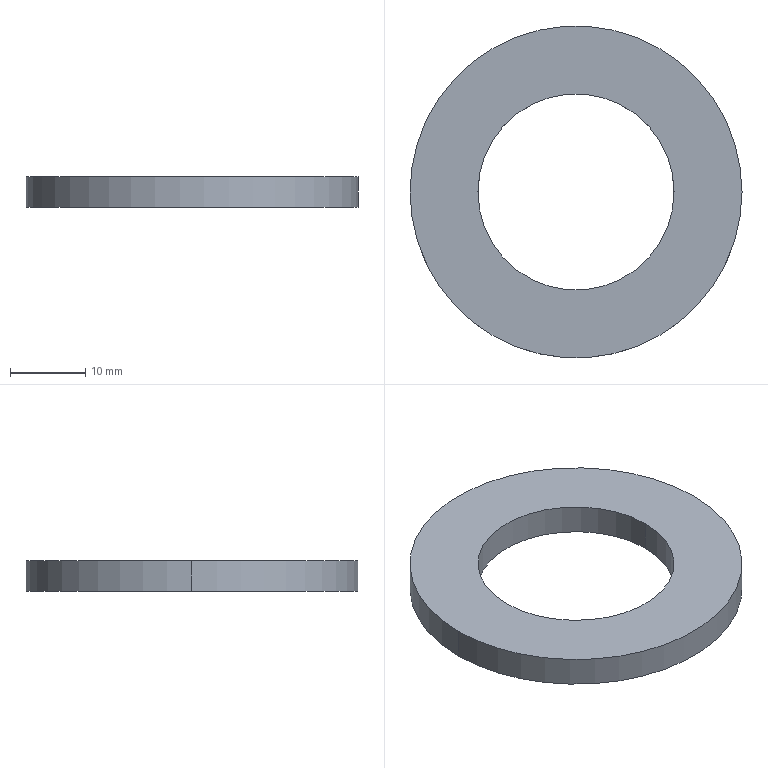Part | SolidWorks | features Extrusion 1 | 1 solid | 6 faces | box 44 x 44 x 4 mm | volume 3958 mm3 | cylinder 4 | plane 2 | commonest cylinder face diameters 26 x2 44 x2
STEP:
#1=CARTESIAN_POINT('',(-13.,0.,-4.));
#2=VERTEX_POINT('',#1);
#3=CARTESIAN_POINT('',(13.,0.,-4.));
#4=VERTEX_POINT('',#3);
#5=CARTESIAN_POINT('',(0.,0.,-4.));
#6=DIRECTION('',(0.,0.,1.));
#7=DIRECTION('',(1.,0.,0.));
#8=AXIS2_PLACEMENT_3D('',#5,#6,#7);
#9=CIRCLE('',#8,13.);
#10=EDGE_CURVE('',#2,#4,#9,.T.);
#11=ORIENTED_EDGE('',*,*,#10,.F.);
#12=CARTESIAN_POINT('',(-13.,0.,0.));
#13=VERTEX_POINT('',#12);
#14=CARTESIAN_POINT('',(-13.,0.,-4.));
#15=DIRECTION('',(0.,0.,1.));
#16=VECTOR('',#15,1000.);
#17=LINE('',#14,#16);
#18=EDGE_CURVE('',#2,#13,#17,.T.);
#19=ORIENTED_EDGE('',*,*,#18,.T.);
#20=CARTESIAN_POINT('',(13.,0.,0.));
#21=VERTEX_POINT('',#20);
#22=CARTESIAN_POINT('',(0.,0.,0.));
#23=DIRECTION('',(0.,0.,1.));
#24=DIRECTION('',(1.,0.,0.));
#25=AXIS2_PLACEMENT_3D('',#22,#23,#24);
#26=CIRCLE('',#25,13.);
#27=EDGE_CURVE('',#13,#21,#26,.T.);
#28=ORIENTED_EDGE('',*,*,#27,.T.);
#29=CARTESIAN_POINT('',(13.,0.,-4.));
#30=DIRECTION('',(0.,0.,1.));
#31=VECTOR('',#30,1000.);
#32=LINE('',#29,#31);
#33=EDGE_CURVE('',#4,#21,#32,.T.);
#34=ORIENTED_EDGE('',*,*,#33,.F.);
#35=EDGE_LOOP('',(#11,#19,#28,#34));
#36=FACE_OUTER_BOUND('',#35,.T.);
#37=CARTESIAN_POINT('',(0.,0.,-4.));
#38=DIRECTION('',(0.,0.,1.));
#39=DIRECTION('',(1.,0.,0.));
#40=AXIS2_PLACEMENT_3D('',#37,#38,#39);
#41=CYLINDRICAL_SURFACE('',#40,13.);
#42=ADVANCED_FACE('',(#36),#41,.F.);
#43=CARTESIAN_POINT('',(22.,0.,-4.));
#44=VERTEX_POINT('',#43);
#45=CARTESIAN_POINT('',(-22.,0.,-4.));
#46=VERTEX_POINT('',#45);
#47=CARTESIAN_POINT('',(0.,0.,-4.));
#48=DIRECTION('',(0.,0.,1.));
#49=DIRECTION('',(1.,0.,0.));
#50=AXIS2_PLACEMENT_3D('',#47,#48,#49);
#51=CIRCLE('',#50,22.);
#52=EDGE_CURVE('',#44,#46,#51,.T.);
#53=ORIENTED_EDGE('',*,*,#52,.T.);
#54=CARTESIAN_POINT('',(-22.,0.,0.));
#55=VERTEX_POINT('',#54);
#56=CARTESIAN_POINT('',(-22.,0.,-4.));
#57=DIRECTION('',(0.,0.,1.));
#58=VECTOR('',#57,1000.);
#59=LINE('',#56,#58);
#60=EDGE_CURVE('',#46,#55,#59,.T.);
#61=ORIENTED_EDGE('',*,*,#60,.T.);
#62=CARTESIAN_POINT('',(22.,0.,0.));
#63=VERTEX_POINT('',#62);
#64=CARTESIAN_POINT('',(0.,0.,0.));
#65=DIRECTION('',(0.,0.,1.));
#66=DIRECTION('',(1.,0.,0.));
#67=AXIS2_PLACEMENT_3D('',#64,#65,#66);
#68=CIRCLE('',#67,22.);
#69=EDGE_CURVE('',#63,#55,#68,.T.);
#70=ORIENTED_EDGE('',*,*,#69,.F.);
#71=CARTESIAN_POINT('',(22.,0.,-4.));
#72=DIRECTION('',(0.,0.,1.));
#73=VECTOR('',#72,1000.);
#74=LINE('',#71,#73);
#75=EDGE_CURVE('',#44,#63,#74,.T.);
#76=ORIENTED_EDGE('',*,*,#75,.F.);
#77=EDGE_LOOP('',(#53,#61,#70,#76));
#78=FACE_OUTER_BOUND('',#77,.T.);
#79=CARTESIAN_POINT('',(0.,0.,-4.));
#80=DIRECTION('',(0.,0.,1.));
#81=DIRECTION('',(1.,0.,0.));
#82=AXIS2_PLACEMENT_3D('',#79,#80,#81);
#83=CYLINDRICAL_SURFACE('',#82,22.);
#84=ADVANCED_FACE('',(#78),#83,.T.);
#85=ORIENTED_EDGE('',*,*,#60,.F.);
#86=CARTESIAN_POINT('',(0.,0.,-4.));
#87=DIRECTION('',(0.,0.,1.));
#88=DIRECTION('',(1.,0.,0.));
#89=AXIS2_PLACEMENT_3D('',#86,#87,#88);
#90=CIRCLE('',#89,22.);
#91=EDGE_CURVE('',#46,#44,#90,.T.);
#92=ORIENTED_EDGE('',*,*,#91,.T.);
#93=ORIENTED_EDGE('',*,*,#75,.T.);
#94=CARTESIAN_POINT('',(0.,0.,0.));
#95=DIRECTION('',(0.,0.,1.));
#96=DIRECTION('',(1.,0.,0.));
#97=AXIS2_PLACEMENT_3D('',#94,#95,#96);
#98=CIRCLE('',#97,22.);
#99=EDGE_CURVE('',#55,#63,#98,.T.);
#100=ORIENTED_EDGE('',*,*,#99,.F.);
#101=EDGE_LOOP('',(#85,#92,#93,#100));
#102=FACE_OUTER_BOUND('',#101,.T.);
#103=CARTESIAN_POINT('',(0.,0.,-4.));
#104=DIRECTION('',(0.,0.,1.));
#105=DIRECTION('',(1.,0.,0.));
#106=AXIS2_PLACEMENT_3D('',#103,#104,#105);
#107=CYLINDRICAL_SURFACE('',#106,22.);
#108=ADVANCED_FACE('',(#102),#107,.T.);
#109=CARTESIAN_POINT('',(0.,0.,-4.));
#110=DIRECTION('',(0.,0.,1.));
#111=DIRECTION('',(1.,0.,0.));
#112=AXIS2_PLACEMENT_3D('',#109,#110,#111);
#113=CIRCLE('',#112,13.);
#114=EDGE_CURVE('',#4,#2,#113,.T.);
#115=ORIENTED_EDGE('',*,*,#114,.T.);
#116=ORIENTED_EDGE('',*,*,#10,.T.);
#117=EDGE_LOOP('',(#115,#116));
#118=FACE_BOUND('',#117,.T.);
#119=ORIENTED_EDGE('',*,*,#52,.F.);
#120=ORIENTED_EDGE('',*,*,#91,.F.);
#121=EDGE_LOOP('',(#119,#120));
#122=FACE_OUTER_BOUND('',#121,.T.);
#123=CARTESIAN_POINT('',(0.,0.,-4.));
#124=DIRECTION('',(0.,0.,1.));
#125=DIRECTION('',(1.,0.,0.));
#126=AXIS2_PLACEMENT_3D('',#123,#124,#125);
#127=PLANE('',#126);
#128=ADVANCED_FACE('',(#118,#122),#127,.F.);
#129=CARTESIAN_POINT('',(0.,0.,0.));
#130=DIRECTION('',(0.,0.,1.));
#131=DIRECTION('',(1.,0.,0.));
#132=AXIS2_PLACEMENT_3D('',#129,#130,#131);
#133=CIRCLE('',#132,13.);
#134=EDGE_CURVE('',#21,#13,#133,.T.);
#135=ORIENTED_EDGE('',*,*,#134,.F.);
#136=ORIENTED_EDGE('',*,*,#27,.F.);
#137=EDGE_LOOP('',(#135,#136));
#138=FACE_BOUND('',#137,.T.);
#139=ORIENTED_EDGE('',*,*,#69,.T.);
#140=ORIENTED_EDGE('',*,*,#99,.T.);
#141=EDGE_LOOP('',(#139,#140));
#142=FACE_OUTER_BOUND('',#141,.T.);
#143=CARTESIAN_POINT('',(0.,0.,0.));
#144=DIRECTION('',(0.,0.,1.));
#145=DIRECTION('',(1.,0.,0.));
#146=AXIS2_PLACEMENT_3D('',#143,#144,#145);
#147=PLANE('',#146);
#148=ADVANCED_FACE('',(#138,#142),#147,.T.);
#149=ORIENTED_EDGE('',*,*,#18,.F.);
#150=ORIENTED_EDGE('',*,*,#114,.F.);
#151=ORIENTED_EDGE('',*,*,#33,.T.);
#152=ORIENTED_EDGE('',*,*,#134,.T.);
#153=EDGE_LOOP('',(#149,#150,#151,#152));
#154=FACE_OUTER_BOUND('',#153,.T.);
#155=CARTESIAN_POINT('',(0.,0.,-4.));
#156=DIRECTION('',(0.,0.,1.));
#157=DIRECTION('',(1.,0.,0.));
#158=AXIS2_PLACEMENT_3D('',#155,#156,#157);
#159=CYLINDRICAL_SURFACE('',#158,13.);
#160=ADVANCED_FACE('',(#154),#159,.F.);
#161=CLOSED_SHELL('',(#42,#84,#108,#128,#148,#160));
#162=MANIFOLD_SOLID_BREP('',#161);
#163=CARTESIAN_POINT('',(0.,0.,0.));
#164=DIRECTION('',(0.,0.,1.));
#165=DIRECTION('',(1.,0.,0.));
#166=AXIS2_PLACEMENT_3D('',#163,#164,#165);
#167=(LENGTH_UNIT()NAMED_UNIT(*)SI_UNIT(.MILLI.,.METRE.));
#168=UNCERTAINTY_MEASURE_WITH_UNIT(LENGTH_MEASURE(0.00001),#167,'','');
#169=(NAMED_UNIT(*)PLANE_ANGLE_UNIT()SI_UNIT($,.RADIAN.));
#170=(NAMED_UNIT(*)SI_UNIT($,.STERADIAN.)SOLID_ANGLE_UNIT());
#171=(GEOMETRIC_REPRESENTATION_CONTEXT(3)GLOBAL_UNCERTAINTY_ASSIGNED_CONTEXT((#168))GLOBAL_UNIT_ASSIGNED_CONTEXT((#167,#169,#170))REPRESENTATION_CONTEXT('',''));
#172=ADVANCED_BREP_SHAPE_REPRESENTATION('',(#162,#166),#171);